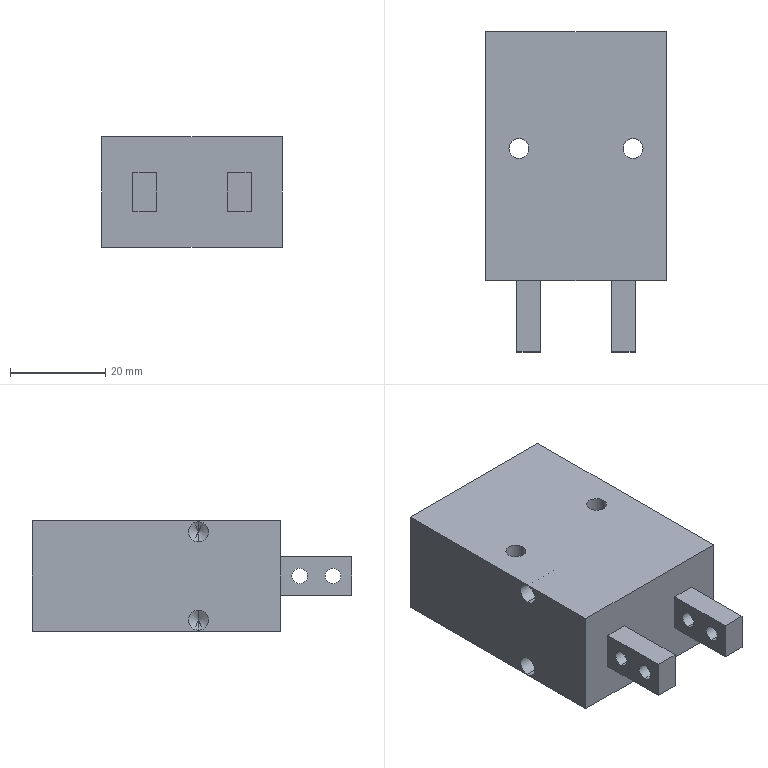Part | 1 solid | 36 faces | box 38 x 67.3 x 23.2 mm | volume 46260 mm3 | cylinder 16 | plane 16 | cone 4 | commonest cylinder face diameters 3.3 x8 4.2 x8
STEP:
#1=CARTESIAN_POINT('',(-9.9,9.15,23.2));
#2=VERTEX_POINT('',#1);
#3=CARTESIAN_POINT('',(-14.1,9.15,23.2));
#4=VERTEX_POINT('',#3);
#5=CARTESIAN_POINT('',(-12.,9.15,23.2));
#6=DIRECTION('',(0.,0.,-1.));
#7=DIRECTION('',(-1.,0.,0.));
#8=AXIS2_PLACEMENT_3D('',#5,#6,#7);
#9=CIRCLE('',#8,2.1);
#10=EDGE_CURVE('',#2,#4,#9,.T.);
#11=ORIENTED_EDGE('',*,*,#10,.F.);
#12=CARTESIAN_POINT('',(-9.9,9.15,0.));
#13=VERTEX_POINT('',#12);
#14=CARTESIAN_POINT('',(-9.9,9.15,0.));
#15=DIRECTION('',(0.,0.,-1.));
#16=VECTOR('',#15,1000.);
#17=LINE('',#14,#16);
#18=EDGE_CURVE('',#2,#13,#17,.T.);
#19=ORIENTED_EDGE('',*,*,#18,.T.);
#20=CARTESIAN_POINT('',(-14.1,9.15,0.));
#21=VERTEX_POINT('',#20);
#22=CARTESIAN_POINT('',(-12.,9.15,0.));
#23=DIRECTION('',(0.,0.,-1.));
#24=DIRECTION('',(-1.,0.,0.));
#25=AXIS2_PLACEMENT_3D('',#22,#23,#24);
#26=CIRCLE('',#25,2.1);
#27=EDGE_CURVE('',#13,#21,#26,.T.);
#28=ORIENTED_EDGE('',*,*,#27,.T.);
#29=CARTESIAN_POINT('',(-14.1,9.15,0.));
#30=DIRECTION('',(0.,0.,-1.));
#31=VECTOR('',#30,1000.);
#32=LINE('',#29,#31);
#33=EDGE_CURVE('',#4,#21,#32,.T.);
#34=ORIENTED_EDGE('',*,*,#33,.F.);
#35=EDGE_LOOP('',(#11,#19,#28,#34));
#36=FACE_OUTER_BOUND('',#35,.T.);
#37=CARTESIAN_POINT('',(-12.,9.15,0.));
#38=DIRECTION('',(0.,0.,-1.));
#39=DIRECTION('',(-1.,0.,0.));
#40=AXIS2_PLACEMENT_3D('',#37,#38,#39);
#41=CYLINDRICAL_SURFACE('',#40,2.1);
#42=ADVANCED_FACE('',(#36),#41,.F.);
#43=CARTESIAN_POINT('',(14.1,9.15,23.2));
#44=VERTEX_POINT('',#43);
#45=CARTESIAN_POINT('',(9.9,9.15,23.2));
#46=VERTEX_POINT('',#45);
#47=CARTESIAN_POINT('',(12.,9.15,23.2));
#48=DIRECTION('',(0.,0.,-1.));
#49=DIRECTION('',(-1.,0.,0.));
#50=AXIS2_PLACEMENT_3D('',#47,#48,#49);
#51=CIRCLE('',#50,2.1);
#52=EDGE_CURVE('',#44,#46,#51,.T.);
#53=ORIENTED_EDGE('',*,*,#52,.F.);
#54=CARTESIAN_POINT('',(14.1,9.15,0.));
#55=VERTEX_POINT('',#54);
#56=CARTESIAN_POINT('',(14.1,9.15,0.));
#57=DIRECTION('',(0.,0.,-1.));
#58=VECTOR('',#57,1000.);
#59=LINE('',#56,#58);
#60=EDGE_CURVE('',#44,#55,#59,.T.);
#61=ORIENTED_EDGE('',*,*,#60,.T.);
#62=CARTESIAN_POINT('',(9.9,9.15,0.));
#63=VERTEX_POINT('',#62);
#64=CARTESIAN_POINT('',(12.,9.15,0.));
#65=DIRECTION('',(0.,0.,-1.));
#66=DIRECTION('',(-1.,0.,0.));
#67=AXIS2_PLACEMENT_3D('',#64,#65,#66);
#68=CIRCLE('',#67,2.1);
#69=EDGE_CURVE('',#55,#63,#68,.T.);
#70=ORIENTED_EDGE('',*,*,#69,.T.);
#71=CARTESIAN_POINT('',(9.9,9.15,0.));
#72=DIRECTION('',(0.,0.,-1.));
#73=VECTOR('',#72,1000.);
#74=LINE('',#71,#73);
#75=EDGE_CURVE('',#46,#63,#74,.T.);
#76=ORIENTED_EDGE('',*,*,#75,.F.);
#77=EDGE_LOOP('',(#53,#61,#70,#76));
#78=FACE_OUTER_BOUND('',#77,.T.);
#79=CARTESIAN_POINT('',(12.,9.15,0.));
#80=DIRECTION('',(0.,0.,-1.));
#81=DIRECTION('',(-1.,0.,0.));
#82=AXIS2_PLACEMENT_3D('',#79,#80,#81);
#83=CYLINDRICAL_SURFACE('',#82,2.1);
#84=ADVANCED_FACE('',(#78),#83,.F.);
#85=CARTESIAN_POINT('',(12.45,-22.65,13.25));
#86=VERTEX_POINT('',#85);
#87=CARTESIAN_POINT('',(12.45,-22.65,9.95));
#88=VERTEX_POINT('',#87);
#89=CARTESIAN_POINT('',(12.45,-22.65,11.6));
#90=DIRECTION('',(1.,0.,0.));
#91=DIRECTION('',(0.,0.,1.));
#92=AXIS2_PLACEMENT_3D('',#89,#90,#91);
#93=CIRCLE('',#92,1.65);
#94=EDGE_CURVE('',#86,#88,#93,.T.);
#95=ORIENTED_EDGE('',*,*,#94,.T.);
#96=CARTESIAN_POINT('',(7.45,-22.65,9.95));
#97=VERTEX_POINT('',#96);
#98=CARTESIAN_POINT('',(-19.,-22.65,9.95));
#99=DIRECTION('',(-1.,0.,0.));
#100=VECTOR('',#99,1000.);
#101=LINE('',#98,#100);
#102=EDGE_CURVE('',#88,#97,#101,.T.);
#103=ORIENTED_EDGE('',*,*,#102,.T.);
#104=CARTESIAN_POINT('',(7.45,-22.65,13.25));
#105=VERTEX_POINT('',#104);
#106=CARTESIAN_POINT('',(7.45,-22.65,11.6));
#107=DIRECTION('',(1.,0.,0.));
#108=DIRECTION('',(0.,0.,-1.));
#109=AXIS2_PLACEMENT_3D('',#106,#107,#108);
#110=CIRCLE('',#109,1.65);
#111=EDGE_CURVE('',#105,#97,#110,.T.);
#112=ORIENTED_EDGE('',*,*,#111,.F.);
#113=CARTESIAN_POINT('',(-19.,-22.65,13.25));
#114=DIRECTION('',(-1.,0.,0.));
#115=VECTOR('',#114,1000.);
#116=LINE('',#113,#115);
#117=EDGE_CURVE('',#86,#105,#116,.T.);
#118=ORIENTED_EDGE('',*,*,#117,.F.);
#119=EDGE_LOOP('',(#95,#103,#112,#118));
#120=FACE_OUTER_BOUND('',#119,.T.);
#121=CARTESIAN_POINT('',(-19.,-22.65,11.6));
#122=DIRECTION('',(-1.,0.,0.));
#123=DIRECTION('',(0.,0.,1.));
#124=AXIS2_PLACEMENT_3D('',#121,#122,#123);
#125=CYLINDRICAL_SURFACE('',#124,1.65);
#126=ADVANCED_FACE('',(#120),#125,.F.);
#127=CARTESIAN_POINT('',(-7.45,-22.65,9.95));
#128=VERTEX_POINT('',#127);
#129=CARTESIAN_POINT('',(-7.45,-22.65,13.25));
#130=VERTEX_POINT('',#129);
#131=CARTESIAN_POINT('',(-7.45,-22.65,11.6));
#132=DIRECTION('',(-1.,0.,0.));
#133=DIRECTION('',(0.,0.,1.));
#134=AXIS2_PLACEMENT_3D('',#131,#132,#133);
#135=CIRCLE('',#134,1.65);
#136=EDGE_CURVE('',#128,#130,#135,.T.);
#137=ORIENTED_EDGE('',*,*,#136,.F.);
#138=CARTESIAN_POINT('',(-12.45,-22.65,9.95));
#139=VERTEX_POINT('',#138);
#140=CARTESIAN_POINT('',(-19.,-22.65,9.95));
#141=DIRECTION('',(-1.,0.,0.));
#142=VECTOR('',#141,1000.);
#143=LINE('',#140,#142);
#144=EDGE_CURVE('',#128,#139,#143,.T.);
#145=ORIENTED_EDGE('',*,*,#144,.T.);
#146=CARTESIAN_POINT('',(-12.45,-22.65,13.25));
#147=VERTEX_POINT('',#146);
#148=CARTESIAN_POINT('',(-12.45,-22.65,11.6));
#149=DIRECTION('',(-1.,0.,0.));
#150=DIRECTION('',(0.,0.,-1.));
#151=AXIS2_PLACEMENT_3D('',#148,#149,#150);
#152=CIRCLE('',#151,1.65);
#153=EDGE_CURVE('',#139,#147,#152,.T.);
#154=ORIENTED_EDGE('',*,*,#153,.T.);
#155=CARTESIAN_POINT('',(-19.,-22.65,13.25));
#156=DIRECTION('',(-1.,0.,0.));
#157=VECTOR('',#156,1000.);
#158=LINE('',#155,#157);
#159=EDGE_CURVE('',#130,#147,#158,.T.);
#160=ORIENTED_EDGE('',*,*,#159,.F.);
#161=EDGE_LOOP('',(#137,#145,#154,#160));
#162=FACE_OUTER_BOUND('',#161,.T.);
#163=CARTESIAN_POINT('',(-19.,-22.65,11.6));
#164=DIRECTION('',(-1.,0.,0.));
#165=DIRECTION('',(0.,0.,1.));
#166=AXIS2_PLACEMENT_3D('',#163,#164,#165);
#167=CYLINDRICAL_SURFACE('',#166,1.65);
#168=ADVANCED_FACE('',(#162),#167,.F.);
#169=CARTESIAN_POINT('',(-7.45,-29.65,9.95));
#170=VERTEX_POINT('',#169);
#171=CARTESIAN_POINT('',(-7.45,-29.65,13.25));
#172=VERTEX_POINT('',#171);
#173=CARTESIAN_POINT('',(-7.45,-29.65,11.6));
#174=DIRECTION('',(-1.,0.,0.));
#175=DIRECTION('',(0.,0.,1.));
#176=AXIS2_PLACEMENT_3D('',#173,#174,#175);
#177=CIRCLE('',#176,1.65);
#178=EDGE_CURVE('',#170,#172,#177,.T.);
#179=ORIENTED_EDGE('',*,*,#178,.F.);
#180=CARTESIAN_POINT('',(-12.45,-29.65,9.95));
#181=VERTEX_POINT('',#180);
#182=CARTESIAN_POINT('',(-19.,-29.65,9.95));
#183=DIRECTION('',(-1.,0.,0.));
#184=VECTOR('',#183,1000.);
#185=LINE('',#182,#184);
#186=EDGE_CURVE('',#170,#181,#185,.T.);
#187=ORIENTED_EDGE('',*,*,#186,.T.);
#188=CARTESIAN_POINT('',(-12.45,-29.65,13.25));
#189=VERTEX_POINT('',#188);
#190=CARTESIAN_POINT('',(-12.45,-29.65,11.6));
#191=DIRECTION('',(-1.,0.,0.));
#192=DIRECTION('',(0.,0.,-1.));
#193=AXIS2_PLACEMENT_3D('',#190,#191,#192);
#194=CIRCLE('',#193,1.65);
#195=EDGE_CURVE('',#181,#189,#194,.T.);
#196=ORIENTED_EDGE('',*,*,#195,.T.);
#197=CARTESIAN_POINT('',(-19.,-29.65,13.25));
#198=DIRECTION('',(-1.,0.,0.));
#199=VECTOR('',#198,1000.);
#200=LINE('',#197,#199);
#201=EDGE_CURVE('',#172,#189,#200,.T.);
#202=ORIENTED_EDGE('',*,*,#201,.F.);
#203=EDGE_LOOP('',(#179,#187,#196,#202));
#204=FACE_OUTER_BOUND('',#203,.T.);
#205=CARTESIAN_POINT('',(-19.,-29.65,11.6));
#206=DIRECTION('',(-1.,0.,0.));
#207=DIRECTION('',(0.,0.,1.));
#208=AXIS2_PLACEMENT_3D('',#205,#206,#207);
#209=CYLINDRICAL_SURFACE('',#208,1.65);
#210=ADVANCED_FACE('',(#204),#209,.F.);
#211=CARTESIAN_POINT('',(12.45,-29.65,13.25));
#212=VERTEX_POINT('',#211);
#213=CARTESIAN_POINT('',(12.45,-29.65,9.95));
#214=VERTEX_POINT('',#213);
#215=CARTESIAN_POINT('',(12.45,-29.65,11.6));
#216=DIRECTION('',(1.,0.,0.));
#217=DIRECTION('',(0.,0.,1.));
#218=AXIS2_PLACEMENT_3D('',#215,#216,#217);
#219=CIRCLE('',#218,1.65);
#220=EDGE_CURVE('',#212,#214,#219,.T.);
#221=ORIENTED_EDGE('',*,*,#220,.T.);
#222=CARTESIAN_POINT('',(7.45,-29.65,9.95));
#223=VERTEX_POINT('',#222);
#224=CARTESIAN_POINT('',(-19.,-29.65,9.95));
#225=DIRECTION('',(-1.,0.,0.));
#226=VECTOR('',#225,1000.);
#227=LINE('',#224,#226);
#228=EDGE_CURVE('',#214,#223,#227,.T.);
#229=ORIENTED_EDGE('',*,*,#228,.T.);
#230=CARTESIAN_POINT('',(7.45,-29.65,13.25));
#231=VERTEX_POINT('',#230);
#232=CARTESIAN_POINT('',(7.45,-29.65,11.6));
#233=DIRECTION('',(1.,0.,0.));
#234=DIRECTION('',(0.,0.,-1.));
#235=AXIS2_PLACEMENT_3D('',#232,#233,#234);
#236=CIRCLE('',#235,1.65);
#237=EDGE_CURVE('',#231,#223,#236,.T.);
#238=ORIENTED_EDGE('',*,*,#237,.F.);
#239=CARTESIAN_POINT('',(-19.,-29.65,13.25));
#240=DIRECTION('',(-1.,0.,0.));
#241=VECTOR('',#240,1000.);
#242=LINE('',#239,#241);
#243=EDGE_CURVE('',#212,#231,#242,.T.);
#244=ORIENTED_EDGE('',*,*,#243,.F.);
#245=EDGE_LOOP('',(#221,#229,#238,#244));
#246=FACE_OUTER_BOUND('',#245,.T.);
#247=CARTESIAN_POINT('',(-19.,-29.65,11.6));
#248=DIRECTION('',(-1.,0.,0.));
#249=DIRECTION('',(0.,0.,1.));
#250=AXIS2_PLACEMENT_3D('',#247,#248,#249);
#251=CYLINDRICAL_SURFACE('',#250,1.65);
#252=ADVANCED_FACE('',(#246),#251,.F.);
#253=CARTESIAN_POINT('',(-11.,-1.35,18.8));
#254=VERTEX_POINT('',#253);
#255=CARTESIAN_POINT('',(-11.,-1.35,23.));
#256=VERTEX_POINT('',#255);
#257=CARTESIAN_POINT('',(-11.,-1.35,20.9));
#258=DIRECTION('',(-1.,0.,0.));
#259=DIRECTION('',(0.,0.,1.));
#260=AXIS2_PLACEMENT_3D('',#257,#258,#259);
#261=CIRCLE('',#260,2.1);
#262=EDGE_CURVE('',#254,#256,#261,.T.);
#263=ORIENTED_EDGE('',*,*,#262,.F.);
#264=CARTESIAN_POINT('',(-19.,-1.35,18.8));
#265=VERTEX_POINT('',#264);
#266=CARTESIAN_POINT('',(-19.,-1.35,18.8));
#267=DIRECTION('',(-1.,0.,0.));
#268=VECTOR('',#267,1000.);
#269=LINE('',#266,#268);
#270=EDGE_CURVE('',#254,#265,#269,.T.);
#271=ORIENTED_EDGE('',*,*,#270,.T.);
#272=CARTESIAN_POINT('',(-19.,-1.35,23.));
#273=VERTEX_POINT('',#272);
#274=CARTESIAN_POINT('',(-19.,-1.35,20.9));
#275=DIRECTION('',(-1.,0.,0.));
#276=DIRECTION('',(0.,0.,1.));
#277=AXIS2_PLACEMENT_3D('',#274,#275,#276);
#278=CIRCLE('',#277,2.1);
#279=EDGE_CURVE('',#265,#273,#278,.T.);
#280=ORIENTED_EDGE('',*,*,#279,.T.);
#281=CARTESIAN_POINT('',(-19.,-1.35,23.));
#282=DIRECTION('',(-1.,0.,0.));
#283=VECTOR('',#282,1000.);
#284=LINE('',#281,#283);
#285=EDGE_CURVE('',#256,#273,#284,.T.);
#286=ORIENTED_EDGE('',*,*,#285,.F.);
#287=EDGE_LOOP('',(#263,#271,#280,#286));
#288=FACE_OUTER_BOUND('',#287,.T.);
#289=CARTESIAN_POINT('',(-19.,-1.35,20.9));
#290=DIRECTION('',(-1.,0.,0.));
#291=DIRECTION('',(0.,0.,1.));
#292=AXIS2_PLACEMENT_3D('',#289,#290,#291);
#293=CYLINDRICAL_SURFACE('',#292,2.1);
#294=ADVANCED_FACE('',(#288),#293,.F.);
#295=CARTESIAN_POINT('',(-9.738,-1.35,20.9));
#296=VERTEX_POINT('',#295);
#297=CARTESIAN_POINT('',(-11.,-1.35,23.));
#298=DIRECTION('',(-0.515,0.,0.8572));
#299=VECTOR('',#298,1000.);
#300=LINE('',#297,#299);
#301=EDGE_CURVE('',#296,#256,#300,.T.);
#302=ORIENTED_EDGE('',*,*,#301,.F.);
#303=CARTESIAN_POINT('',(-11.,-1.35,18.8));
#304=DIRECTION('',(-0.515,0.,-0.8572));
#305=VECTOR('',#304,1000.);
#306=LINE('',#303,#305);
#307=EDGE_CURVE('',#296,#254,#306,.T.);
#308=ORIENTED_EDGE('',*,*,#307,.T.);
#309=ORIENTED_EDGE('',*,*,#262,.T.);
#310=EDGE_LOOP('',(#302,#308,#309));
#311=FACE_OUTER_BOUND('',#310,.T.);
#312=CARTESIAN_POINT('',(-11.,-1.35,20.9));
#313=DIRECTION('',(-1.,0.,0.));
#314=DIRECTION('',(0.,0.,1.));
#315=AXIS2_PLACEMENT_3D('',#312,#313,#314);
#316=CONICAL_SURFACE('',#315,2.1,1.03);
#317=ADVANCED_FACE('',(#311),#316,.F.);
#318=CARTESIAN_POINT('',(-11.,-1.35,0.2));
#319=VERTEX_POINT('',#318);
#320=CARTESIAN_POINT('',(-11.,-1.35,4.4));
#321=VERTEX_POINT('',#320);
#322=CARTESIAN_POINT('',(-11.,-1.35,2.3));
#323=DIRECTION('',(-1.,0.,0.));
#324=DIRECTION('',(0.,0.,1.));
#325=AXIS2_PLACEMENT_3D('',#322,#323,#324);
#326=CIRCLE('',#325,2.1);
#327=EDGE_CURVE('',#319,#321,#326,.T.);
#328=ORIENTED_EDGE('',*,*,#327,.F.);
#329=CARTESIAN_POINT('',(-19.,-1.35,0.2));
#330=VERTEX_POINT('',#329);
#331=CARTESIAN_POINT('',(-19.,-1.35,0.2));
#332=DIRECTION('',(-1.,0.,0.));
#333=VECTOR('',#332,1000.);
#334=LINE('',#331,#333);
#335=EDGE_CURVE('',#319,#330,#334,.T.);
#336=ORIENTED_EDGE('',*,*,#335,.T.);
#337=CARTESIAN_POINT('',(-19.,-1.35,4.4));
#338=VERTEX_POINT('',#337);
#339=CARTESIAN_POINT('',(-19.,-1.35,2.3));
#340=DIRECTION('',(-1.,0.,0.));
#341=DIRECTION('',(0.,0.,1.));
#342=AXIS2_PLACEMENT_3D('',#339,#340,#341);
#343=CIRCLE('',#342,2.1);
#344=EDGE_CURVE('',#330,#338,#343,.T.);
#345=ORIENTED_EDGE('',*,*,#344,.T.);
#346=CARTESIAN_POINT('',(-19.,-1.35,4.4));
#347=DIRECTION('',(-1.,0.,0.));
#348=VECTOR('',#347,1000.);
#349=LINE('',#346,#348);
#350=EDGE_CURVE('',#321,#338,#349,.T.);
#351=ORIENTED_EDGE('',*,*,#350,.F.);
#352=EDGE_LOOP('',(#328,#336,#345,#351));
#353=FACE_OUTER_BOUND('',#352,.T.);
#354=CARTESIAN_POINT('',(-19.,-1.35,2.3));
#355=DIRECTION('',(-1.,0.,0.));
#356=DIRECTION('',(0.,0.,1.));
#357=AXIS2_PLACEMENT_3D('',#354,#355,#356);
#358=CYLINDRICAL_SURFACE('',#357,2.1);
#359=ADVANCED_FACE('',(#353),#358,.F.);
#360=CARTESIAN_POINT('',(-9.738,-1.35,2.3));
#361=VERTEX_POINT('',#360);
#362=CARTESIAN_POINT('',(-11.,-1.35,4.4));
#363=DIRECTION('',(-0.515,0.,0.8572));
#364=VECTOR('',#363,1000.);
#365=LINE('',#362,#364);
#366=EDGE_CURVE('',#361,#321,#365,.T.);
#367=ORIENTED_EDGE('',*,*,#366,.F.);
#368=CARTESIAN_POINT('',(-11.,-1.35,0.2));
#369=DIRECTION('',(-0.515,0.,-0.8572));
#370=VECTOR('',#369,1000.);
#371=LINE('',#368,#370);
#372=EDGE_CURVE('',#361,#319,#371,.T.);
#373=ORIENTED_EDGE('',*,*,#372,.T.);
#374=ORIENTED_EDGE('',*,*,#327,.T.);
#375=EDGE_LOOP('',(#367,#373,#374));
#376=FACE_OUTER_BOUND('',#375,.T.);
#377=CARTESIAN_POINT('',(-11.,-1.35,2.3));
#378=DIRECTION('',(-1.,0.,0.));
#379=DIRECTION('',(0.,0.,1.));
#380=AXIS2_PLACEMENT_3D('',#377,#378,#379);
#381=CONICAL_SURFACE('',#380,2.1,1.03);
#382=ADVANCED_FACE('',(#376),#381,.F.);
#383=CARTESIAN_POINT('',(-19.,-1.35,2.3));
#384=DIRECTION('',(-1.,0.,0.));
#385=DIRECTION('',(0.,0.,1.));
#386=AXIS2_PLACEMENT_3D('',#383,#384,#385);
#387=CIRCLE('',#386,2.1);
#388=EDGE_CURVE('',#338,#330,#387,.T.);
#389=ORIENTED_EDGE('',*,*,#388,.F.);
#390=ORIENTED_EDGE('',*,*,#344,.F.);
#391=EDGE_LOOP('',(#389,#390));
#392=FACE_BOUND('',#391,.T.);
#393=CARTESIAN_POINT('',(-19.,33.65,0.));
#394=VERTEX_POINT('',#393);
#395=CARTESIAN_POINT('',(-19.,-18.65,0.));
#396=VERTEX_POINT('',#395);
#397=CARTESIAN_POINT('',(-19.,-33.65,0.));
#398=DIRECTION('',(0.,-1.,0.));
#399=VECTOR('',#398,1000.);
#400=LINE('',#397,#399);
#401=EDGE_CURVE('',#394,#396,#400,.T.);
#402=ORIENTED_EDGE('',*,*,#401,.T.);
#403=CARTESIAN_POINT('',(-19.,-18.65,23.2));
#404=VERTEX_POINT('',#403);
#405=CARTESIAN_POINT('',(-19.,-18.65,23.2));
#406=DIRECTION('',(0.,0.,-1.));
#407=VECTOR('',#406,1000.);
#408=LINE('',#405,#407);
#409=EDGE_CURVE('',#404,#396,#408,.T.);
#410=ORIENTED_EDGE('',*,*,#409,.F.);
#411=CARTESIAN_POINT('',(-19.,33.65,23.2));
#412=VERTEX_POINT('',#411);
#413=CARTESIAN_POINT('',(-19.,-33.65,23.2));
#414=DIRECTION('',(0.,-1.,0.));
#415=VECTOR('',#414,1000.);
#416=LINE('',#413,#415);
#417=EDGE_CURVE('',#412,#404,#416,.T.);
#418=ORIENTED_EDGE('',*,*,#417,.F.);
#419=CARTESIAN_POINT('',(-19.,33.65,23.2));
#420=DIRECTION('',(0.,0.,-1.));
#421=VECTOR('',#420,1000.);
#422=LINE('',#419,#421);
#423=EDGE_CURVE('',#412,#394,#422,.T.);
#424=ORIENTED_EDGE('',*,*,#423,.T.);
#425=EDGE_LOOP('',(#402,#410,#418,#424));
#426=FACE_OUTER_BOUND('',#425,.T.);
#427=CARTESIAN_POINT('',(-19.,-1.35,20.9));
#428=DIRECTION('',(-1.,0.,0.));
#429=DIRECTION('',(0.,0.,1.));
#430=AXIS2_PLACEMENT_3D('',#427,#428,#429);
#431=CIRCLE('',#430,2.1);
#432=EDGE_CURVE('',#273,#265,#431,.T.);
#433=ORIENTED_EDGE('',*,*,#432,.F.);
#434=ORIENTED_EDGE('',*,*,#279,.F.);
#435=EDGE_LOOP('',(#433,#434));
#436=FACE_BOUND('',#435,.T.);
#437=CARTESIAN_POINT('',(-19.,-33.65,23.2));
#438=DIRECTION('',(1.,0.,0.));
#439=DIRECTION('',(0.,0.,-1.));
#440=AXIS2_PLACEMENT_3D('',#437,#438,#439);
#441=PLANE('',#440);
#442=ADVANCED_FACE('',(#392,#426,#436),#441,.F.);
#443=CARTESIAN_POINT('',(-12.,9.15,0.));
#444=DIRECTION('',(0.,0.,-1.));
#445=DIRECTION('',(-1.,0.,0.));
#446=AXIS2_PLACEMENT_3D('',#443,#444,#445);
#447=CIRCLE('',#446,2.1);
#448=EDGE_CURVE('',#21,#13,#447,.T.);
#449=ORIENTED_EDGE('',*,*,#448,.F.);
#450=ORIENTED_EDGE('',*,*,#27,.F.);
#451=EDGE_LOOP('',(#449,#450));
#452=FACE_BOUND('',#451,.T.);
#453=CARTESIAN_POINT('',(12.,9.15,0.));
#454=DIRECTION('',(0.,0.,-1.));
#455=DIRECTION('',(-1.,0.,0.));
#456=AXIS2_PLACEMENT_3D('',#453,#454,#455);
#457=CIRCLE('',#456,2.1);
#458=EDGE_CURVE('',#63,#55,#457,.T.);
#459=ORIENTED_EDGE('',*,*,#458,.F.);
#460=ORIENTED_EDGE('',*,*,#69,.F.);
#461=EDGE_LOOP('',(#459,#460));
#462=FACE_BOUND('',#461,.T.);
#463=CARTESIAN_POINT('',(19.,-18.65,0.));
#464=VERTEX_POINT('',#463);
#465=CARTESIAN_POINT('',(19.,33.65,0.));
#466=VERTEX_POINT('',#465);
#467=CARTESIAN_POINT('',(19.,-33.65,0.));
#468=DIRECTION('',(0.,1.,0.));
#469=VECTOR('',#468,1000.);
#470=LINE('',#467,#469);
#471=EDGE_CURVE('',#464,#466,#470,.T.);
#472=ORIENTED_EDGE('',*,*,#471,.F.);
#473=CARTESIAN_POINT('',(0.,-18.65,0.));
#474=DIRECTION('',(1.,0.,0.));
#475=VECTOR('',#474,1000.);
#476=LINE('',#473,#475);
#477=EDGE_CURVE('',#396,#464,#476,.T.);
#478=ORIENTED_EDGE('',*,*,#477,.F.);
#479=ORIENTED_EDGE('',*,*,#401,.F.);
#480=CARTESIAN_POINT('',(-19.,33.65,0.));
#481=DIRECTION('',(-1.,0.,0.));
#482=VECTOR('',#481,1000.);
#483=LINE('',#480,#482);
#484=EDGE_CURVE('',#466,#394,#483,.T.);
#485=ORIENTED_EDGE('',*,*,#484,.F.);
#486=EDGE_LOOP('',(#472,#478,#479,#485));
#487=FACE_OUTER_BOUND('',#486,.T.);
#488=CARTESIAN_POINT('',(0.,0.,0.));
#489=DIRECTION('',(0.,0.,-1.));
#490=DIRECTION('',(-1.,0.,0.));
#491=AXIS2_PLACEMENT_3D('',#488,#489,#490);
#492=PLANE('',#491);
#493=ADVANCED_FACE('',(#452,#462,#487),#492,.T.);
#494=CARTESIAN_POINT('',(-12.,9.15,23.2));
#495=DIRECTION('',(0.,0.,-1.));
#496=DIRECTION('',(-1.,0.,0.));
#497=AXIS2_PLACEMENT_3D('',#494,#495,#496);
#498=CIRCLE('',#497,2.1);
#499=EDGE_CURVE('',#4,#2,#498,.T.);
#500=ORIENTED_EDGE('',*,*,#499,.T.);
#501=ORIENTED_EDGE('',*,*,#10,.T.);
#502=EDGE_LOOP('',(#500,#501));
#503=FACE_BOUND('',#502,.T.);
#504=CARTESIAN_POINT('',(12.,9.15,23.2));
#505=DIRECTION('',(0.,0.,-1.));
#506=DIRECTION('',(-1.,0.,0.));
#507=AXIS2_PLACEMENT_3D('',#504,#505,#506);
#508=CIRCLE('',#507,2.1);
#509=EDGE_CURVE('',#46,#44,#508,.T.);
#510=ORIENTED_EDGE('',*,*,#509,.T.);
#511=ORIENTED_EDGE('',*,*,#52,.T.);
#512=EDGE_LOOP('',(#510,#511));
#513=FACE_BOUND('',#512,.T.);
#514=CARTESIAN_POINT('',(19.,-18.65,23.2));
#515=VERTEX_POINT('',#514);
#516=CARTESIAN_POINT('',(-7.45,-18.65,23.2));
#517=DIRECTION('',(-1.,0.,0.));
#518=VECTOR('',#517,1000.);
#519=LINE('',#516,#518);
#520=EDGE_CURVE('',#515,#404,#519,.T.);
#521=ORIENTED_EDGE('',*,*,#520,.F.);
#522=CARTESIAN_POINT('',(19.,33.65,23.2));
#523=VERTEX_POINT('',#522);
#524=CARTESIAN_POINT('',(19.,-33.65,23.2));
#525=DIRECTION('',(0.,1.,0.));
#526=VECTOR('',#525,1000.);
#527=LINE('',#524,#526);
#528=EDGE_CURVE('',#515,#523,#527,.T.);
#529=ORIENTED_EDGE('',*,*,#528,.T.);
#530=CARTESIAN_POINT('',(-19.,33.65,23.2));
#531=DIRECTION('',(-1.,0.,0.));
#532=VECTOR('',#531,1000.);
#533=LINE('',#530,#532);
#534=EDGE_CURVE('',#523,#412,#533,.T.);
#535=ORIENTED_EDGE('',*,*,#534,.T.);
#536=ORIENTED_EDGE('',*,*,#417,.T.);
#537=EDGE_LOOP('',(#521,#529,#535,#536));
#538=FACE_OUTER_BOUND('',#537,.T.);
#539=CARTESIAN_POINT('',(0.,0.,23.2));
#540=DIRECTION('',(0.,0.,-1.));
#541=DIRECTION('',(-1.,0.,0.));
#542=AXIS2_PLACEMENT_3D('',#539,#540,#541);
#543=PLANE('',#542);
#544=ADVANCED_FACE('',(#503,#513,#538),#543,.F.);
#545=CARTESIAN_POINT('',(12.45,-33.65,7.6));
#546=VERTEX_POINT('',#545);
#547=CARTESIAN_POINT('',(7.45,-33.65,7.6));
#548=VERTEX_POINT('',#547);
#549=CARTESIAN_POINT('',(19.,-33.65,7.6));
#550=DIRECTION('',(-1.,0.,0.));
#551=VECTOR('',#550,1000.);
#552=LINE('',#549,#551);
#553=EDGE_CURVE('',#546,#548,#552,.T.);
#554=ORIENTED_EDGE('',*,*,#553,.F.);
#555=CARTESIAN_POINT('',(12.45,-33.65,15.6));
#556=VERTEX_POINT('',#555);
#557=CARTESIAN_POINT('',(12.45,-33.65,29.54));
#558=DIRECTION('',(0.,0.,-1.));
#559=VECTOR('',#558,1000.);
#560=LINE('',#557,#559);
#561=EDGE_CURVE('',#556,#546,#560,.T.);
#562=ORIENTED_EDGE('',*,*,#561,.F.);
#563=CARTESIAN_POINT('',(7.45,-33.65,15.6));
#564=VERTEX_POINT('',#563);
#565=CARTESIAN_POINT('',(-19.,-33.65,15.6));
#566=DIRECTION('',(1.,0.,0.));
#567=VECTOR('',#566,1000.);
#568=LINE('',#565,#567);
#569=EDGE_CURVE('',#564,#556,#568,.T.);
#570=ORIENTED_EDGE('',*,*,#569,.F.);
#571=CARTESIAN_POINT('',(7.45,-33.65,-3.523));
#572=DIRECTION('',(0.,0.,1.));
#573=VECTOR('',#572,1000.);
#574=LINE('',#571,#573);
#575=EDGE_CURVE('',#548,#564,#574,.T.);
#576=ORIENTED_EDGE('',*,*,#575,.F.);
#577=EDGE_LOOP('',(#554,#562,#570,#576));
#578=FACE_OUTER_BOUND('',#577,.T.);
#579=CARTESIAN_POINT('',(-19.,-33.65,23.2));
#580=DIRECTION('',(0.,1.,0.));
#581=DIRECTION('',(0.,0.,1.));
#582=AXIS2_PLACEMENT_3D('',#579,#580,#581);
#583=PLANE('',#582);
#584=ADVANCED_FACE('',(#578),#583,.F.);
#585=CARTESIAN_POINT('',(19.,-18.65,23.2));
#586=DIRECTION('',(0.,0.,1.));
#587=VECTOR('',#586,1000.);
#588=LINE('',#585,#587);
#589=EDGE_CURVE('',#464,#515,#588,.T.);
#590=ORIENTED_EDGE('',*,*,#589,.F.);
#591=ORIENTED_EDGE('',*,*,#471,.T.);
#592=CARTESIAN_POINT('',(19.,33.65,23.2));
#593=DIRECTION('',(0.,0.,-1.));
#594=VECTOR('',#593,1000.);
#595=LINE('',#592,#594);
#596=EDGE_CURVE('',#523,#466,#595,.T.);
#597=ORIENTED_EDGE('',*,*,#596,.F.);
#598=ORIENTED_EDGE('',*,*,#528,.F.);
#599=EDGE_LOOP('',(#590,#591,#597,#598));
#600=FACE_OUTER_BOUND('',#599,.T.);
#601=CARTESIAN_POINT('',(19.,-33.65,23.2));
#602=DIRECTION('',(-1.,0.,0.));
#603=DIRECTION('',(0.,0.,1.));
#604=AXIS2_PLACEMENT_3D('',#601,#602,#603);
#605=PLANE('',#604);
#606=ADVANCED_FACE('',(#600),#605,.F.);
#607=ORIENTED_EDGE('',*,*,#484,.T.);
#608=ORIENTED_EDGE('',*,*,#423,.F.);
#609=ORIENTED_EDGE('',*,*,#534,.F.);
#610=ORIENTED_EDGE('',*,*,#596,.T.);
#611=EDGE_LOOP('',(#607,#608,#609,#610));
#612=FACE_OUTER_BOUND('',#611,.T.);
#613=CARTESIAN_POINT('',(-19.,33.65,23.2));
#614=DIRECTION('',(0.,-1.,0.));
#615=DIRECTION('',(0.,0.,-1.));
#616=AXIS2_PLACEMENT_3D('',#613,#614,#615);
#617=PLANE('',#616);
#618=ADVANCED_FACE('',(#612),#617,.F.);
#619=CARTESIAN_POINT('',(-12.45,-33.65,15.6));
#620=VERTEX_POINT('',#619);
#621=CARTESIAN_POINT('',(-7.45,-33.65,15.6));
#622=VERTEX_POINT('',#621);
#623=CARTESIAN_POINT('',(-19.,-33.65,15.6));
#624=DIRECTION('',(1.,0.,0.));
#625=VECTOR('',#624,1000.);
#626=LINE('',#623,#625);
#627=EDGE_CURVE('',#620,#622,#626,.T.);
#628=ORIENTED_EDGE('',*,*,#627,.F.);
#629=CARTESIAN_POINT('',(-12.45,-33.65,7.6));
#630=VERTEX_POINT('',#629);
#631=CARTESIAN_POINT('',(-12.45,-33.65,25.898));
#632=DIRECTION('',(0.,0.,1.));
#633=VECTOR('',#632,1000.);
#634=LINE('',#631,#633);
#635=EDGE_CURVE('',#630,#620,#634,.T.);
#636=ORIENTED_EDGE('',*,*,#635,.F.);
#637=CARTESIAN_POINT('',(-7.45,-33.65,7.6));
#638=VERTEX_POINT('',#637);
#639=CARTESIAN_POINT('',(19.,-33.65,7.6));
#640=DIRECTION('',(-1.,0.,0.));
#641=VECTOR('',#640,1000.);
#642=LINE('',#639,#641);
#643=EDGE_CURVE('',#638,#630,#642,.T.);
#644=ORIENTED_EDGE('',*,*,#643,.F.);
#645=CARTESIAN_POINT('',(-7.45,-33.65,-3.523));
#646=DIRECTION('',(0.,0.,-1.));
#647=VECTOR('',#646,1000.);
#648=LINE('',#645,#647);
#649=EDGE_CURVE('',#622,#638,#648,.T.);
#650=ORIENTED_EDGE('',*,*,#649,.F.);
#651=EDGE_LOOP('',(#628,#636,#644,#650));
#652=FACE_OUTER_BOUND('',#651,.T.);
#653=CARTESIAN_POINT('',(-19.,-33.65,23.2));
#654=DIRECTION('',(0.,1.,0.));
#655=DIRECTION('',(0.,0.,1.));
#656=AXIS2_PLACEMENT_3D('',#653,#654,#655);
#657=PLANE('',#656);
#658=ADVANCED_FACE('',(#652),#657,.F.);
#659=ORIENTED_EDGE('',*,*,#111,.T.);
#660=CARTESIAN_POINT('',(7.45,-22.65,11.6));
#661=DIRECTION('',(1.,0.,0.));
#662=DIRECTION('',(0.,0.,-1.));
#663=AXIS2_PLACEMENT_3D('',#660,#661,#662);
#664=CIRCLE('',#663,1.65);
#665=EDGE_CURVE('',#97,#105,#664,.T.);
#666=ORIENTED_EDGE('',*,*,#665,.T.);
#667=EDGE_LOOP('',(#659,#666));
#668=FACE_BOUND('',#667,.T.);
#669=ORIENTED_EDGE('',*,*,#237,.T.);
#670=CARTESIAN_POINT('',(7.45,-29.65,11.6));
#671=DIRECTION('',(1.,0.,0.));
#672=DIRECTION('',(0.,0.,-1.));
#673=AXIS2_PLACEMENT_3D('',#670,#671,#672);
#674=CIRCLE('',#673,1.65);
#675=EDGE_CURVE('',#223,#231,#674,.T.);
#676=ORIENTED_EDGE('',*,*,#675,.T.);
#677=EDGE_LOOP('',(#669,#676));
#678=FACE_BOUND('',#677,.T.);
#679=CARTESIAN_POINT('',(7.45,-18.65,7.6));
#680=VERTEX_POINT('',#679);
#681=CARTESIAN_POINT('',(7.45,-18.65,15.6));
#682=VERTEX_POINT('',#681);
#683=CARTESIAN_POINT('',(7.45,-18.65,-3.523));
#684=DIRECTION('',(0.,0.,1.));
#685=VECTOR('',#684,1000.);
#686=LINE('',#683,#685);
#687=EDGE_CURVE('',#680,#682,#686,.T.);
#688=ORIENTED_EDGE('',*,*,#687,.F.);
#689=CARTESIAN_POINT('',(7.45,-18.65,7.6));
#690=DIRECTION('',(0.,-1.,0.));
#691=VECTOR('',#690,1000.);
#692=LINE('',#689,#691);
#693=EDGE_CURVE('',#680,#548,#692,.T.);
#694=ORIENTED_EDGE('',*,*,#693,.T.);
#695=ORIENTED_EDGE('',*,*,#575,.T.);
#696=CARTESIAN_POINT('',(7.45,-18.65,15.6));
#697=DIRECTION('',(0.,1.,0.));
#698=VECTOR('',#697,1000.);
#699=LINE('',#696,#698);
#700=EDGE_CURVE('',#564,#682,#699,.T.);
#701=ORIENTED_EDGE('',*,*,#700,.T.);
#702=EDGE_LOOP('',(#688,#694,#695,#701));
#703=FACE_OUTER_BOUND('',#702,.T.);
#704=CARTESIAN_POINT('',(7.45,-18.65,-3.523));
#705=DIRECTION('',(1.,0.,0.));
#706=DIRECTION('',(0.,0.,-1.));
#707=AXIS2_PLACEMENT_3D('',#704,#705,#706);
#708=PLANE('',#707);
#709=ADVANCED_FACE('',(#668,#678,#703),#708,.F.);
#710=CARTESIAN_POINT('',(-7.45,-22.65,11.6));
#711=DIRECTION('',(-1.,0.,0.));
#712=DIRECTION('',(0.,0.,1.));
#713=AXIS2_PLACEMENT_3D('',#710,#711,#712);
#714=CIRCLE('',#713,1.65);
#715=EDGE_CURVE('',#130,#128,#714,.T.);
#716=ORIENTED_EDGE('',*,*,#715,.T.);
#717=ORIENTED_EDGE('',*,*,#136,.T.);
#718=EDGE_LOOP('',(#716,#717));
#719=FACE_BOUND('',#718,.T.);
#720=CARTESIAN_POINT('',(-7.45,-29.65,11.6));
#721=DIRECTION('',(-1.,0.,0.));
#722=DIRECTION('',(0.,0.,1.));
#723=AXIS2_PLACEMENT_3D('',#720,#721,#722);
#724=CIRCLE('',#723,1.65);
#725=EDGE_CURVE('',#172,#170,#724,.T.);
#726=ORIENTED_EDGE('',*,*,#725,.T.);
#727=ORIENTED_EDGE('',*,*,#178,.T.);
#728=EDGE_LOOP('',(#726,#727));
#729=FACE_BOUND('',#728,.T.);
#730=ORIENTED_EDGE('',*,*,#649,.T.);
#731=CARTESIAN_POINT('',(-7.45,-18.65,7.6));
#732=VERTEX_POINT('',#731);
#733=CARTESIAN_POINT('',(-7.45,-18.65,7.6));
#734=DIRECTION('',(0.,1.,0.));
#735=VECTOR('',#734,1000.);
#736=LINE('',#733,#735);
#737=EDGE_CURVE('',#638,#732,#736,.T.);
#738=ORIENTED_EDGE('',*,*,#737,.T.);
#739=CARTESIAN_POINT('',(-7.45,-18.65,15.6));
#740=VERTEX_POINT('',#739);
#741=CARTESIAN_POINT('',(-7.45,-18.65,-3.523));
#742=DIRECTION('',(0.,0.,-1.));
#743=VECTOR('',#742,1000.);
#744=LINE('',#741,#743);
#745=EDGE_CURVE('',#740,#732,#744,.T.);
#746=ORIENTED_EDGE('',*,*,#745,.F.);
#747=CARTESIAN_POINT('',(-7.45,-18.65,15.6));
#748=DIRECTION('',(0.,-1.,0.));
#749=VECTOR('',#748,1000.);
#750=LINE('',#747,#749);
#751=EDGE_CURVE('',#740,#622,#750,.T.);
#752=ORIENTED_EDGE('',*,*,#751,.T.);
#753=EDGE_LOOP('',(#730,#738,#746,#752));
#754=FACE_OUTER_BOUND('',#753,.T.);
#755=CARTESIAN_POINT('',(-7.45,-18.65,-3.523));
#756=DIRECTION('',(-1.,0.,0.));
#757=DIRECTION('',(0.,0.,1.));
#758=AXIS2_PLACEMENT_3D('',#755,#756,#757);
#759=PLANE('',#758);
#760=ADVANCED_FACE('',(#719,#729,#754),#759,.F.);
#761=CARTESIAN_POINT('',(12.45,-18.65,15.6));
#762=VERTEX_POINT('',#761);
#763=CARTESIAN_POINT('',(12.45,-18.65,7.6));
#764=VERTEX_POINT('',#763);
#765=CARTESIAN_POINT('',(12.45,-18.65,29.54));
#766=DIRECTION('',(0.,0.,-1.));
#767=VECTOR('',#766,1000.);
#768=LINE('',#765,#767);
#769=EDGE_CURVE('',#762,#764,#768,.T.);
#770=ORIENTED_EDGE('',*,*,#769,.T.);
#771=CARTESIAN_POINT('',(19.,-18.65,7.6));
#772=DIRECTION('',(-1.,0.,0.));
#773=VECTOR('',#772,1000.);
#774=LINE('',#771,#773);
#775=EDGE_CURVE('',#764,#680,#774,.T.);
#776=ORIENTED_EDGE('',*,*,#775,.T.);
#777=ORIENTED_EDGE('',*,*,#687,.T.);
#778=CARTESIAN_POINT('',(-19.,-18.65,15.6));
#779=DIRECTION('',(1.,0.,0.));
#780=VECTOR('',#779,1000.);
#781=LINE('',#778,#780);
#782=EDGE_CURVE('',#682,#762,#781,.T.);
#783=ORIENTED_EDGE('',*,*,#782,.T.);
#784=EDGE_LOOP('',(#770,#776,#777,#783));
#785=FACE_BOUND('',#784,.T.);
#786=CARTESIAN_POINT('',(-12.45,-18.65,7.6));
#787=VERTEX_POINT('',#786);
#788=CARTESIAN_POINT('',(-12.45,-18.65,15.6));
#789=VERTEX_POINT('',#788);
#790=CARTESIAN_POINT('',(-12.45,-18.65,25.898));
#791=DIRECTION('',(0.,0.,1.));
#792=VECTOR('',#791,1000.);
#793=LINE('',#790,#792);
#794=EDGE_CURVE('',#787,#789,#793,.T.);
#795=ORIENTED_EDGE('',*,*,#794,.T.);
#796=CARTESIAN_POINT('',(-19.,-18.65,15.6));
#797=DIRECTION('',(1.,0.,0.));
#798=VECTOR('',#797,1000.);
#799=LINE('',#796,#798);
#800=EDGE_CURVE('',#789,#740,#799,.T.);
#801=ORIENTED_EDGE('',*,*,#800,.T.);
#802=ORIENTED_EDGE('',*,*,#745,.T.);
#803=CARTESIAN_POINT('',(19.,-18.65,7.6));
#804=DIRECTION('',(-1.,0.,0.));
#805=VECTOR('',#804,1000.);
#806=LINE('',#803,#805);
#807=EDGE_CURVE('',#732,#787,#806,.T.);
#808=ORIENTED_EDGE('',*,*,#807,.T.);
#809=EDGE_LOOP('',(#795,#801,#802,#808));
#810=FACE_BOUND('',#809,.T.);
#811=ORIENTED_EDGE('',*,*,#477,.T.);
#812=ORIENTED_EDGE('',*,*,#589,.T.);
#813=ORIENTED_EDGE('',*,*,#520,.T.);
#814=ORIENTED_EDGE('',*,*,#409,.T.);
#815=EDGE_LOOP('',(#811,#812,#813,#814));
#816=FACE_OUTER_BOUND('',#815,.T.);
#817=CARTESIAN_POINT('',(0.,-18.65,0.));
#818=DIRECTION('',(0.,1.,0.));
#819=DIRECTION('',(0.,0.,1.));
#820=AXIS2_PLACEMENT_3D('',#817,#818,#819);
#821=PLANE('',#820);
#822=ADVANCED_FACE('',(#785,#810,#816),#821,.F.);
#823=ORIENTED_EDGE('',*,*,#800,.F.);
#824=CARTESIAN_POINT('',(-12.45,-18.65,15.6));
#825=DIRECTION('',(0.,-1.,0.));
#826=VECTOR('',#825,1000.);
#827=LINE('',#824,#826);
#828=EDGE_CURVE('',#789,#620,#827,.T.);
#829=ORIENTED_EDGE('',*,*,#828,.T.);
#830=ORIENTED_EDGE('',*,*,#627,.T.);
#831=ORIENTED_EDGE('',*,*,#751,.F.);
#832=EDGE_LOOP('',(#823,#829,#830,#831));
#833=FACE_OUTER_BOUND('',#832,.T.);
#834=CARTESIAN_POINT('',(-19.,-18.65,15.6));
#835=DIRECTION('',(0.,0.,-1.));
#836=DIRECTION('',(-1.,0.,0.));
#837=AXIS2_PLACEMENT_3D('',#834,#835,#836);
#838=PLANE('',#837);
#839=ADVANCED_FACE('',(#833),#838,.F.);
#840=ORIENTED_EDGE('',*,*,#569,.T.);
#841=CARTESIAN_POINT('',(12.45,-18.65,15.6));
#842=DIRECTION('',(0.,1.,0.));
#843=VECTOR('',#842,1000.);
#844=LINE('',#841,#843);
#845=EDGE_CURVE('',#556,#762,#844,.T.);
#846=ORIENTED_EDGE('',*,*,#845,.T.);
#847=ORIENTED_EDGE('',*,*,#782,.F.);
#848=ORIENTED_EDGE('',*,*,#700,.F.);
#849=EDGE_LOOP('',(#840,#846,#847,#848));
#850=FACE_OUTER_BOUND('',#849,.T.);
#851=CARTESIAN_POINT('',(-19.,-18.65,15.6));
#852=DIRECTION('',(0.,0.,-1.));
#853=DIRECTION('',(-1.,0.,0.));
#854=AXIS2_PLACEMENT_3D('',#851,#852,#853);
#855=PLANE('',#854);
#856=ADVANCED_FACE('',(#850),#855,.F.);
#857=ORIENTED_EDGE('',*,*,#643,.T.);
#858=CARTESIAN_POINT('',(-12.45,-18.65,7.6));
#859=DIRECTION('',(0.,1.,0.));
#860=VECTOR('',#859,1000.);
#861=LINE('',#858,#860);
#862=EDGE_CURVE('',#630,#787,#861,.T.);
#863=ORIENTED_EDGE('',*,*,#862,.T.);
#864=ORIENTED_EDGE('',*,*,#807,.F.);
#865=ORIENTED_EDGE('',*,*,#737,.F.);
#866=EDGE_LOOP('',(#857,#863,#864,#865));
#867=FACE_OUTER_BOUND('',#866,.T.);
#868=CARTESIAN_POINT('',(19.,-18.65,7.6));
#869=DIRECTION('',(0.,0.,1.));
#870=DIRECTION('',(1.,0.,0.));
#871=AXIS2_PLACEMENT_3D('',#868,#869,#870);
#872=PLANE('',#871);
#873=ADVANCED_FACE('',(#867),#872,.F.);
#874=ORIENTED_EDGE('',*,*,#775,.F.);
#875=CARTESIAN_POINT('',(12.45,-18.65,7.6));
#876=DIRECTION('',(0.,-1.,0.));
#877=VECTOR('',#876,1000.);
#878=LINE('',#875,#877);
#879=EDGE_CURVE('',#764,#546,#878,.T.);
#880=ORIENTED_EDGE('',*,*,#879,.T.);
#881=ORIENTED_EDGE('',*,*,#553,.T.);
#882=ORIENTED_EDGE('',*,*,#693,.F.);
#883=EDGE_LOOP('',(#874,#880,#881,#882));
#884=FACE_OUTER_BOUND('',#883,.T.);
#885=CARTESIAN_POINT('',(19.,-18.65,7.6));
#886=DIRECTION('',(0.,0.,1.));
#887=DIRECTION('',(1.,0.,0.));
#888=AXIS2_PLACEMENT_3D('',#885,#886,#887);
#889=PLANE('',#888);
#890=ADVANCED_FACE('',(#884),#889,.F.);
#891=ORIENTED_EDGE('',*,*,#372,.F.);
#892=ORIENTED_EDGE('',*,*,#366,.T.);
#893=CARTESIAN_POINT('',(-11.,-1.35,2.3));
#894=DIRECTION('',(-1.,0.,0.));
#895=DIRECTION('',(0.,0.,1.));
#896=AXIS2_PLACEMENT_3D('',#893,#894,#895);
#897=CIRCLE('',#896,2.1);
#898=EDGE_CURVE('',#321,#319,#897,.T.);
#899=ORIENTED_EDGE('',*,*,#898,.T.);
#900=EDGE_LOOP('',(#891,#892,#899));
#901=FACE_OUTER_BOUND('',#900,.T.);
#902=CARTESIAN_POINT('',(-11.,-1.35,2.3));
#903=DIRECTION('',(-1.,0.,0.));
#904=DIRECTION('',(0.,0.,1.));
#905=AXIS2_PLACEMENT_3D('',#902,#903,#904);
#906=CONICAL_SURFACE('',#905,2.1,1.03);
#907=ADVANCED_FACE('',(#901),#906,.F.);
#908=ORIENTED_EDGE('',*,*,#335,.F.);
#909=ORIENTED_EDGE('',*,*,#898,.F.);
#910=ORIENTED_EDGE('',*,*,#350,.T.);
#911=ORIENTED_EDGE('',*,*,#388,.T.);
#912=EDGE_LOOP('',(#908,#909,#910,#911));
#913=FACE_OUTER_BOUND('',#912,.T.);
#914=CARTESIAN_POINT('',(-19.,-1.35,2.3));
#915=DIRECTION('',(-1.,0.,0.));
#916=DIRECTION('',(0.,0.,1.));
#917=AXIS2_PLACEMENT_3D('',#914,#915,#916);
#918=CYLINDRICAL_SURFACE('',#917,2.1);
#919=ADVANCED_FACE('',(#913),#918,.F.);
#920=ORIENTED_EDGE('',*,*,#307,.F.);
#921=ORIENTED_EDGE('',*,*,#301,.T.);
#922=CARTESIAN_POINT('',(-11.,-1.35,20.9));
#923=DIRECTION('',(-1.,0.,0.));
#924=DIRECTION('',(0.,0.,1.));
#925=AXIS2_PLACEMENT_3D('',#922,#923,#924);
#926=CIRCLE('',#925,2.1);
#927=EDGE_CURVE('',#256,#254,#926,.T.);
#928=ORIENTED_EDGE('',*,*,#927,.T.);
#929=EDGE_LOOP('',(#920,#921,#928));
#930=FACE_OUTER_BOUND('',#929,.T.);
#931=CARTESIAN_POINT('',(-11.,-1.35,20.9));
#932=DIRECTION('',(-1.,0.,0.));
#933=DIRECTION('',(0.,0.,1.));
#934=AXIS2_PLACEMENT_3D('',#931,#932,#933);
#935=CONICAL_SURFACE('',#934,2.1,1.03);
#936=ADVANCED_FACE('',(#930),#935,.F.);
#937=ORIENTED_EDGE('',*,*,#270,.F.);
#938=ORIENTED_EDGE('',*,*,#927,.F.);
#939=ORIENTED_EDGE('',*,*,#285,.T.);
#940=ORIENTED_EDGE('',*,*,#432,.T.);
#941=EDGE_LOOP('',(#937,#938,#939,#940));
#942=FACE_OUTER_BOUND('',#941,.T.);
#943=CARTESIAN_POINT('',(-19.,-1.35,20.9));
#944=DIRECTION('',(-1.,0.,0.));
#945=DIRECTION('',(0.,0.,1.));
#946=AXIS2_PLACEMENT_3D('',#943,#944,#945);
#947=CYLINDRICAL_SURFACE('',#946,2.1);
#948=ADVANCED_FACE('',(#942),#947,.F.);
#949=ORIENTED_EDGE('',*,*,#228,.F.);
#950=CARTESIAN_POINT('',(12.45,-29.65,11.6));
#951=DIRECTION('',(1.,0.,0.));
#952=DIRECTION('',(0.,0.,1.));
#953=AXIS2_PLACEMENT_3D('',#950,#951,#952);
#954=CIRCLE('',#953,1.65);
#955=EDGE_CURVE('',#214,#212,#954,.T.);
#956=ORIENTED_EDGE('',*,*,#955,.T.);
#957=ORIENTED_EDGE('',*,*,#243,.T.);
#958=ORIENTED_EDGE('',*,*,#675,.F.);
#959=EDGE_LOOP('',(#949,#956,#957,#958));
#960=FACE_OUTER_BOUND('',#959,.T.);
#961=CARTESIAN_POINT('',(-19.,-29.65,11.6));
#962=DIRECTION('',(-1.,0.,0.));
#963=DIRECTION('',(0.,0.,1.));
#964=AXIS2_PLACEMENT_3D('',#961,#962,#963);
#965=CYLINDRICAL_SURFACE('',#964,1.65);
#966=ADVANCED_FACE('',(#960),#965,.F.);
#967=ORIENTED_EDGE('',*,*,#186,.F.);
#968=ORIENTED_EDGE('',*,*,#725,.F.);
#969=ORIENTED_EDGE('',*,*,#201,.T.);
#970=CARTESIAN_POINT('',(-12.45,-29.65,11.6));
#971=DIRECTION('',(-1.,0.,0.));
#972=DIRECTION('',(0.,0.,-1.));
#973=AXIS2_PLACEMENT_3D('',#970,#971,#972);
#974=CIRCLE('',#973,1.65);
#975=EDGE_CURVE('',#189,#181,#974,.T.);
#976=ORIENTED_EDGE('',*,*,#975,.T.);
#977=EDGE_LOOP('',(#967,#968,#969,#976));
#978=FACE_OUTER_BOUND('',#977,.T.);
#979=CARTESIAN_POINT('',(-19.,-29.65,11.6));
#980=DIRECTION('',(-1.,0.,0.));
#981=DIRECTION('',(0.,0.,1.));
#982=AXIS2_PLACEMENT_3D('',#979,#980,#981);
#983=CYLINDRICAL_SURFACE('',#982,1.65);
#984=ADVANCED_FACE('',(#978),#983,.F.);
#985=ORIENTED_EDGE('',*,*,#144,.F.);
#986=ORIENTED_EDGE('',*,*,#715,.F.);
#987=ORIENTED_EDGE('',*,*,#159,.T.);
#988=CARTESIAN_POINT('',(-12.45,-22.65,11.6));
#989=DIRECTION('',(-1.,0.,0.));
#990=DIRECTION('',(0.,0.,-1.));
#991=AXIS2_PLACEMENT_3D('',#988,#989,#990);
#992=CIRCLE('',#991,1.65);
#993=EDGE_CURVE('',#147,#139,#992,.T.);
#994=ORIENTED_EDGE('',*,*,#993,.T.);
#995=EDGE_LOOP('',(#985,#986,#987,#994));
#996=FACE_OUTER_BOUND('',#995,.T.);
#997=CARTESIAN_POINT('',(-19.,-22.65,11.6));
#998=DIRECTION('',(-1.,0.,0.));
#999=DIRECTION('',(0.,0.,1.));
#1000=AXIS2_PLACEMENT_3D('',#997,#998,#999);
#1001=CYLINDRICAL_SURFACE('',#1000,1.65);
#1002=ADVANCED_FACE('',(#996),#1001,.F.);
#1003=ORIENTED_EDGE('',*,*,#102,.F.);
#1004=CARTESIAN_POINT('',(12.45,-22.65,11.6));
#1005=DIRECTION('',(1.,0.,0.));
#1006=DIRECTION('',(0.,0.,1.));
#1007=AXIS2_PLACEMENT_3D('',#1004,#1005,#1006);
#1008=CIRCLE('',#1007,1.65);
#1009=EDGE_CURVE('',#88,#86,#1008,.T.);
#1010=ORIENTED_EDGE('',*,*,#1009,.T.);
#1011=ORIENTED_EDGE('',*,*,#117,.T.);
#1012=ORIENTED_EDGE('',*,*,#665,.F.);
#1013=EDGE_LOOP('',(#1003,#1010,#1011,#1012));
#1014=FACE_OUTER_BOUND('',#1013,.T.);
#1015=CARTESIAN_POINT('',(-19.,-22.65,11.6));
#1016=DIRECTION('',(-1.,0.,0.));
#1017=DIRECTION('',(0.,0.,1.));
#1018=AXIS2_PLACEMENT_3D('',#1015,#1016,#1017);
#1019=CYLINDRICAL_SURFACE('',#1018,1.65);
#1020=ADVANCED_FACE('',(#1014),#1019,.F.);
#1021=ORIENTED_EDGE('',*,*,#60,.F.);
#1022=ORIENTED_EDGE('',*,*,#509,.F.);
#1023=ORIENTED_EDGE('',*,*,#75,.T.);
#1024=ORIENTED_EDGE('',*,*,#458,.T.);
#1025=EDGE_LOOP('',(#1021,#1022,#1023,#1024));
#1026=FACE_OUTER_BOUND('',#1025,.T.);
#1027=CARTESIAN_POINT('',(12.,9.15,0.));
#1028=DIRECTION('',(0.,0.,-1.));
#1029=DIRECTION('',(-1.,0.,0.));
#1030=AXIS2_PLACEMENT_3D('',#1027,#1028,#1029);
#1031=CYLINDRICAL_SURFACE('',#1030,2.1);
#1032=ADVANCED_FACE('',(#1026),#1031,.F.);
#1033=ORIENTED_EDGE('',*,*,#18,.F.);
#1034=ORIENTED_EDGE('',*,*,#499,.F.);
#1035=ORIENTED_EDGE('',*,*,#33,.T.);
#1036=ORIENTED_EDGE('',*,*,#448,.T.);
#1037=EDGE_LOOP('',(#1033,#1034,#1035,#1036));
#1038=FACE_OUTER_BOUND('',#1037,.T.);
#1039=CARTESIAN_POINT('',(-12.,9.15,0.));
#1040=DIRECTION('',(0.,0.,-1.));
#1041=DIRECTION('',(-1.,0.,0.));
#1042=AXIS2_PLACEMENT_3D('',#1039,#1040,#1041);
#1043=CYLINDRICAL_SURFACE('',#1042,2.1);
#1044=ADVANCED_FACE('',(#1038),#1043,.F.);
#1045=ORIENTED_EDGE('',*,*,#993,.F.);
#1046=ORIENTED_EDGE('',*,*,#153,.F.);
#1047=EDGE_LOOP('',(#1045,#1046));
#1048=FACE_BOUND('',#1047,.T.);
#1049=ORIENTED_EDGE('',*,*,#975,.F.);
#1050=ORIENTED_EDGE('',*,*,#195,.F.);
#1051=EDGE_LOOP('',(#1049,#1050));
#1052=FACE_BOUND('',#1051,.T.);
#1053=ORIENTED_EDGE('',*,*,#794,.F.);
#1054=ORIENTED_EDGE('',*,*,#862,.F.);
#1055=ORIENTED_EDGE('',*,*,#635,.T.);
#1056=ORIENTED_EDGE('',*,*,#828,.F.);
#1057=EDGE_LOOP('',(#1053,#1054,#1055,#1056));
#1058=FACE_OUTER_BOUND('',#1057,.T.);
#1059=CARTESIAN_POINT('',(-12.45,18.718,25.898));
#1060=DIRECTION('',(1.,0.,0.));
#1061=DIRECTION('',(0.,0.,-1.));
#1062=AXIS2_PLACEMENT_3D('',#1059,#1060,#1061);
#1063=PLANE('',#1062);
#1064=ADVANCED_FACE('',(#1048,#1052,#1058),#1063,.F.);
#1065=ORIENTED_EDGE('',*,*,#94,.F.);
#1066=ORIENTED_EDGE('',*,*,#1009,.F.);
#1067=EDGE_LOOP('',(#1065,#1066));
#1068=FACE_BOUND('',#1067,.T.);
#1069=ORIENTED_EDGE('',*,*,#220,.F.);
#1070=ORIENTED_EDGE('',*,*,#955,.F.);
#1071=EDGE_LOOP('',(#1069,#1070));
#1072=FACE_BOUND('',#1071,.T.);
#1073=ORIENTED_EDGE('',*,*,#561,.T.);
#1074=ORIENTED_EDGE('',*,*,#879,.F.);
#1075=ORIENTED_EDGE('',*,*,#769,.F.);
#1076=ORIENTED_EDGE('',*,*,#845,.F.);
#1077=EDGE_LOOP('',(#1073,#1074,#1075,#1076));
#1078=FACE_OUTER_BOUND('',#1077,.T.);
#1079=CARTESIAN_POINT('',(12.45,18.718,29.54));
#1080=DIRECTION('',(-1.,0.,0.));
#1081=DIRECTION('',(0.,0.,1.));
#1082=AXIS2_PLACEMENT_3D('',#1079,#1080,#1081);
#1083=PLANE('',#1082);
#1084=ADVANCED_FACE('',(#1068,#1072,#1078),#1083,.F.);
#1085=CLOSED_SHELL('',(#42,#84,#126,#168,#210,#252,#294,#317,#359,#382,#442,#493,#544,#584,#606,#618,#658,#709,#760,#822,#839,#856,#873,#890,#907,#919,#936,#948,#966,#984,#1002,#1020,#1032,#1044,#1064,#1084));
#1086=MANIFOLD_SOLID_BREP('',#1085);
#1087=CARTESIAN_POINT('',(0.,0.,0.));
#1088=DIRECTION('',(0.,0.,1.));
#1089=DIRECTION('',(1.,0.,0.));
#1090=AXIS2_PLACEMENT_3D('',#1087,#1088,#1089);
#1091=(LENGTH_UNIT()NAMED_UNIT(*)SI_UNIT(.MILLI.,.METRE.));
#1092=UNCERTAINTY_MEASURE_WITH_UNIT(LENGTH_MEASURE(0.00001),#1091,'','');
#1093=(NAMED_UNIT(*)PLANE_ANGLE_UNIT()SI_UNIT($,.RADIAN.));
#1094=(NAMED_UNIT(*)SI_UNIT($,.STERADIAN.)SOLID_ANGLE_UNIT());
#1095=(GEOMETRIC_REPRESENTATION_CONTEXT(3)GLOBAL_UNCERTAINTY_ASSIGNED_CONTEXT((#1092))GLOBAL_UNIT_ASSIGNED_CONTEXT((#1091,#1093,#1094))REPRESENTATION_CONTEXT('',''));
#1096=ADVANCED_BREP_SHAPE_REPRESENTATION('',(#1086,#1090),#1095);